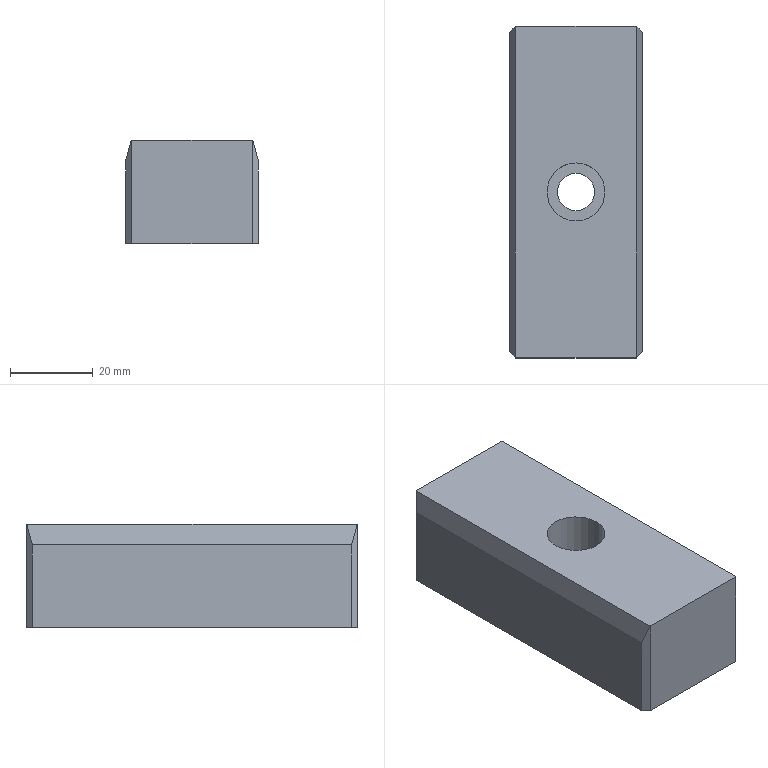Part | NX | features solid 2 | 1 solid | 15 faces | box 32 x 80 x 25 mm | volume 60691 mm3 | plane 13 | cylinder 2 | commonest cylinder face diameters 9 x1 14 x1
STEP:
#1=CARTESIAN_POINT('',(465.,749.5,-145.));
#2=VERTEX_POINT('',#1);
#3=CARTESIAN_POINT('',(465.,745.,-145.));
#4=DIRECTION('',(0.,0.,-1.));
#5=DIRECTION('',(0.,1.,0.));
#6=AXIS2_PLACEMENT_3D('',#3,#4,#5);
#7=CIRCLE('',#6,4.5);
#8=EDGE_CURVE('',#2,#2,#7,.F.);
#9=ORIENTED_EDGE('',*,*,#8,.F.);
#10=EDGE_LOOP('',(#9));
#11=FACE_BOUND('',#10,.T.);
#12=CARTESIAN_POINT('',(465.,740.5,-132.));
#13=VERTEX_POINT('',#12);
#14=CARTESIAN_POINT('',(465.,745.,-132.));
#15=DIRECTION('',(0.,0.,1.));
#16=DIRECTION('',(0.,-1.,0.));
#17=AXIS2_PLACEMENT_3D('',#14,#15,#16);
#18=CIRCLE('',#17,4.5);
#19=EDGE_CURVE('',#13,#13,#18,.T.);
#20=ORIENTED_EDGE('',*,*,#19,.T.);
#21=EDGE_LOOP('',(#20));
#22=FACE_BOUND('',#21,.T.);
#23=CARTESIAN_POINT('',(465.,745.,-70.));
#24=DIRECTION('',(0.,0.,-1.));
#25=DIRECTION('',(0.,1.,0.));
#26=AXIS2_PLACEMENT_3D('',#23,#24,#25);
#27=CYLINDRICAL_SURFACE('',#26,4.5);
#28=ADVANCED_FACE('',(#11,#22),#27,.F.);
#29=CARTESIAN_POINT('',(479.5,705.,-145.));
#30=VERTEX_POINT('',#29);
#31=CARTESIAN_POINT('',(450.5,705.,-145.));
#32=VERTEX_POINT('',#31);
#33=CARTESIAN_POINT('',(481.,705.,-145.));
#34=DIRECTION('',(-1.,0.,0.));
#35=VECTOR('',#34,1000.);
#36=LINE('',#33,#35);
#37=EDGE_CURVE('',#30,#32,#36,.T.);
#38=ORIENTED_EDGE('',*,*,#37,.T.);
#39=CARTESIAN_POINT('',(449.,706.5,-145.));
#40=VERTEX_POINT('',#39);
#41=CARTESIAN_POINT('',(425.75,729.75,-145.));
#42=DIRECTION('',(0.7071,-0.7071,0.));
#43=VECTOR('',#42,1000.);
#44=LINE('',#41,#43);
#45=EDGE_CURVE('',#32,#40,#44,.F.);
#46=ORIENTED_EDGE('',*,*,#45,.T.);
#47=CARTESIAN_POINT('',(449.,783.5,-145.));
#48=VERTEX_POINT('',#47);
#49=CARTESIAN_POINT('',(449.,705.,-145.));
#50=DIRECTION('',(0.,1.,0.));
#51=VECTOR('',#50,1000.);
#52=LINE('',#49,#51);
#53=EDGE_CURVE('',#40,#48,#52,.T.);
#54=ORIENTED_EDGE('',*,*,#53,.T.);
#55=CARTESIAN_POINT('',(450.5,785.,-145.));
#56=VERTEX_POINT('',#55);
#57=CARTESIAN_POINT('',(465.75,800.25,-145.));
#58=DIRECTION('',(-0.7071,-0.7071,0.));
#59=VECTOR('',#58,1000.);
#60=LINE('',#57,#59);
#61=EDGE_CURVE('',#48,#56,#60,.F.);
#62=ORIENTED_EDGE('',*,*,#61,.T.);
#63=CARTESIAN_POINT('',(479.5,785.,-145.));
#64=VERTEX_POINT('',#63);
#65=CARTESIAN_POINT('',(449.,785.,-145.));
#66=DIRECTION('',(1.,0.,0.));
#67=VECTOR('',#66,1000.);
#68=LINE('',#65,#67);
#69=EDGE_CURVE('',#56,#64,#68,.T.);
#70=ORIENTED_EDGE('',*,*,#69,.T.);
#71=CARTESIAN_POINT('',(481.,783.5,-145.));
#72=VERTEX_POINT('',#71);
#73=CARTESIAN_POINT('',(480.25,784.25,-145.));
#74=DIRECTION('',(-0.7071,0.7071,0.));
#75=VECTOR('',#74,1000.);
#76=LINE('',#73,#75);
#77=EDGE_CURVE('',#64,#72,#76,.F.);
#78=ORIENTED_EDGE('',*,*,#77,.T.);
#79=CARTESIAN_POINT('',(481.,706.5,-145.));
#80=VERTEX_POINT('',#79);
#81=CARTESIAN_POINT('',(481.,785.,-145.));
#82=DIRECTION('',(0.,-1.,0.));
#83=VECTOR('',#82,1000.);
#84=LINE('',#81,#83);
#85=EDGE_CURVE('',#72,#80,#84,.T.);
#86=ORIENTED_EDGE('',*,*,#85,.T.);
#87=CARTESIAN_POINT('',(520.25,745.75,-145.));
#88=DIRECTION('',(0.7071,0.7071,0.));
#89=VECTOR('',#88,1000.);
#90=LINE('',#87,#89);
#91=EDGE_CURVE('',#80,#30,#90,.F.);
#92=ORIENTED_EDGE('',*,*,#91,.T.);
#93=EDGE_LOOP('',(#38,#46,#54,#62,#70,#78,#86,#92));
#94=FACE_BOUND('',#93,.T.);
#95=ORIENTED_EDGE('',*,*,#8,.T.);
#96=EDGE_LOOP('',(#95));
#97=FACE_BOUND('',#96,.T.);
#98=CARTESIAN_POINT('',(481.,785.,-145.));
#99=DIRECTION('',(0.,0.,-1.));
#100=DIRECTION('',(0.,1.,0.));
#101=AXIS2_PLACEMENT_3D('',#98,#99,#100);
#102=PLANE('',#101);
#103=ADVANCED_FACE('',(#94,#97),#102,.T.);
#104=CARTESIAN_POINT('',(465.,738.,-120.));
#105=VERTEX_POINT('',#104);
#106=CARTESIAN_POINT('',(465.,745.,-120.));
#107=DIRECTION('',(0.,0.,1.));
#108=DIRECTION('',(0.,-1.,0.));
#109=AXIS2_PLACEMENT_3D('',#106,#107,#108);
#110=CIRCLE('',#109,7.);
#111=EDGE_CURVE('',#105,#105,#110,.T.);
#112=ORIENTED_EDGE('',*,*,#111,.F.);
#113=EDGE_LOOP('',(#112));
#114=FACE_BOUND('',#113,.T.);
#115=CARTESIAN_POINT('',(450.5,785.,-120.));
#116=VERTEX_POINT('',#115);
#117=CARTESIAN_POINT('',(450.34,784.84,-120.));
#118=VERTEX_POINT('',#117);
#119=CARTESIAN_POINT('',(450.5,785.,-120.));
#120=DIRECTION('',(0.7071,0.7071,0.));
#121=VECTOR('',#120,1000.);
#122=LINE('',#119,#121);
#123=EDGE_CURVE('',#116,#118,#122,.F.);
#124=ORIENTED_EDGE('',*,*,#123,.T.);
#125=CARTESIAN_POINT('',(450.34,705.16,-120.));
#126=VERTEX_POINT('',#125);
#127=CARTESIAN_POINT('',(450.34,785.,-120.));
#128=DIRECTION('',(0.,-1.,0.));
#129=VECTOR('',#128,1000.);
#130=LINE('',#127,#129);
#131=EDGE_CURVE('',#118,#126,#130,.T.);
#132=ORIENTED_EDGE('',*,*,#131,.T.);
#133=CARTESIAN_POINT('',(450.5,705.,-120.));
#134=VERTEX_POINT('',#133);
#135=CARTESIAN_POINT('',(449.,706.5,-120.));
#136=DIRECTION('',(-0.7071,0.7071,0.));
#137=VECTOR('',#136,1000.);
#138=LINE('',#135,#137);
#139=EDGE_CURVE('',#126,#134,#138,.F.);
#140=ORIENTED_EDGE('',*,*,#139,.T.);
#141=CARTESIAN_POINT('',(479.5,705.,-120.));
#142=VERTEX_POINT('',#141);
#143=CARTESIAN_POINT('',(481.,705.,-120.));
#144=DIRECTION('',(-1.,0.,0.));
#145=VECTOR('',#144,1000.);
#146=LINE('',#143,#145);
#147=EDGE_CURVE('',#142,#134,#146,.T.);
#148=ORIENTED_EDGE('',*,*,#147,.F.);
#149=CARTESIAN_POINT('',(479.66,705.16,-120.));
#150=VERTEX_POINT('',#149);
#151=CARTESIAN_POINT('',(479.5,705.,-120.));
#152=DIRECTION('',(-0.7071,-0.7071,0.));
#153=VECTOR('',#152,1000.);
#154=LINE('',#151,#153);
#155=EDGE_CURVE('',#142,#150,#154,.F.);
#156=ORIENTED_EDGE('',*,*,#155,.T.);
#157=CARTESIAN_POINT('',(479.66,784.84,-120.));
#158=VERTEX_POINT('',#157);
#159=CARTESIAN_POINT('',(479.66,785.,-120.));
#160=DIRECTION('',(0.,1.,0.));
#161=VECTOR('',#160,1000.);
#162=LINE('',#159,#161);
#163=EDGE_CURVE('',#150,#158,#162,.T.);
#164=ORIENTED_EDGE('',*,*,#163,.T.);
#165=CARTESIAN_POINT('',(479.5,785.,-120.));
#166=VERTEX_POINT('',#165);
#167=CARTESIAN_POINT('',(481.,783.5,-120.));
#168=DIRECTION('',(0.7071,-0.7071,0.));
#169=VECTOR('',#168,1000.);
#170=LINE('',#167,#169);
#171=EDGE_CURVE('',#158,#166,#170,.F.);
#172=ORIENTED_EDGE('',*,*,#171,.T.);
#173=CARTESIAN_POINT('',(449.,785.,-120.));
#174=DIRECTION('',(1.,0.,0.));
#175=VECTOR('',#174,1000.);
#176=LINE('',#173,#175);
#177=EDGE_CURVE('',#116,#166,#176,.T.);
#178=ORIENTED_EDGE('',*,*,#177,.F.);
#179=EDGE_LOOP('',(#124,#132,#140,#148,#156,#164,#172,#178));
#180=FACE_BOUND('',#179,.T.);
#181=CARTESIAN_POINT('',(481.,785.,-120.));
#182=DIRECTION('',(0.,0.,-1.));
#183=DIRECTION('',(0.,1.,0.));
#184=AXIS2_PLACEMENT_3D('',#181,#182,#183);
#185=PLANE('',#184);
#186=ADVANCED_FACE('',(#114,#180),#185,.F.);
#187=ORIENTED_EDGE('',*,*,#69,.F.);
#188=CARTESIAN_POINT('',(450.5,785.,-145.));
#189=DIRECTION('',(0.,0.,1.));
#190=VECTOR('',#189,1000.);
#191=LINE('',#188,#190);
#192=EDGE_CURVE('',#56,#116,#191,.T.);
#193=ORIENTED_EDGE('',*,*,#192,.T.);
#194=ORIENTED_EDGE('',*,*,#177,.T.);
#195=CARTESIAN_POINT('',(479.5,785.,-145.));
#196=DIRECTION('',(0.,0.,-1.));
#197=VECTOR('',#196,1000.);
#198=LINE('',#195,#197);
#199=EDGE_CURVE('',#166,#64,#198,.T.);
#200=ORIENTED_EDGE('',*,*,#199,.T.);
#201=EDGE_LOOP('',(#187,#193,#194,#200));
#202=FACE_BOUND('',#201,.T.);
#203=CARTESIAN_POINT('',(449.,785.,-145.));
#204=DIRECTION('',(0.,-1.,0.));
#205=DIRECTION('',(0.,0.,-1.));
#206=AXIS2_PLACEMENT_3D('',#203,#204,#205);
#207=PLANE('',#206);
#208=ADVANCED_FACE('',(#202),#207,.F.);
#209=CARTESIAN_POINT('',(481.,783.5,-125.));
#210=VERTEX_POINT('',#209);
#211=CARTESIAN_POINT('',(481.,783.5,-145.));
#212=DIRECTION('',(0.,0.,1.));
#213=VECTOR('',#212,1000.);
#214=LINE('',#211,#213);
#215=EDGE_CURVE('',#72,#210,#214,.T.);
#216=ORIENTED_EDGE('',*,*,#215,.T.);
#217=CARTESIAN_POINT('',(481.,706.5,-125.));
#218=VERTEX_POINT('',#217);
#219=CARTESIAN_POINT('',(481.,785.,-125.));
#220=DIRECTION('',(0.,-1.,0.));
#221=VECTOR('',#220,1000.);
#222=LINE('',#219,#221);
#223=EDGE_CURVE('',#210,#218,#222,.T.);
#224=ORIENTED_EDGE('',*,*,#223,.T.);
#225=CARTESIAN_POINT('',(481.,706.5,-145.));
#226=DIRECTION('',(0.,0.,-1.));
#227=VECTOR('',#226,1000.);
#228=LINE('',#225,#227);
#229=EDGE_CURVE('',#218,#80,#228,.T.);
#230=ORIENTED_EDGE('',*,*,#229,.T.);
#231=ORIENTED_EDGE('',*,*,#85,.F.);
#232=EDGE_LOOP('',(#216,#224,#230,#231));
#233=FACE_BOUND('',#232,.T.);
#234=CARTESIAN_POINT('',(481.,785.,-145.));
#235=DIRECTION('',(-1.,0.,0.));
#236=DIRECTION('',(0.,0.,-1.));
#237=AXIS2_PLACEMENT_3D('',#234,#235,#236);
#238=PLANE('',#237);
#239=ADVANCED_FACE('',(#233),#238,.F.);
#240=ORIENTED_EDGE('',*,*,#147,.T.);
#241=CARTESIAN_POINT('',(450.5,705.,-145.));
#242=DIRECTION('',(0.,0.,-1.));
#243=VECTOR('',#242,1000.);
#244=LINE('',#241,#243);
#245=EDGE_CURVE('',#134,#32,#244,.T.);
#246=ORIENTED_EDGE('',*,*,#245,.T.);
#247=ORIENTED_EDGE('',*,*,#37,.F.);
#248=CARTESIAN_POINT('',(479.5,705.,-145.));
#249=DIRECTION('',(0.,0.,1.));
#250=VECTOR('',#249,1000.);
#251=LINE('',#248,#250);
#252=EDGE_CURVE('',#30,#142,#251,.T.);
#253=ORIENTED_EDGE('',*,*,#252,.T.);
#254=EDGE_LOOP('',(#240,#246,#247,#253));
#255=FACE_BOUND('',#254,.T.);
#256=CARTESIAN_POINT('',(481.,705.,-145.));
#257=DIRECTION('',(0.,1.,0.));
#258=DIRECTION('',(0.,0.,1.));
#259=AXIS2_PLACEMENT_3D('',#256,#257,#258);
#260=PLANE('',#259);
#261=ADVANCED_FACE('',(#255),#260,.F.);
#262=CARTESIAN_POINT('',(449.,706.5,-125.));
#263=VERTEX_POINT('',#262);
#264=CARTESIAN_POINT('',(449.,706.5,-145.));
#265=DIRECTION('',(0.,0.,1.));
#266=VECTOR('',#265,1000.);
#267=LINE('',#264,#266);
#268=EDGE_CURVE('',#40,#263,#267,.T.);
#269=ORIENTED_EDGE('',*,*,#268,.T.);
#270=CARTESIAN_POINT('',(449.,783.5,-125.));
#271=VERTEX_POINT('',#270);
#272=CARTESIAN_POINT('',(449.,705.,-125.));
#273=DIRECTION('',(0.,1.,0.));
#274=VECTOR('',#273,1000.);
#275=LINE('',#272,#274);
#276=EDGE_CURVE('',#263,#271,#275,.T.);
#277=ORIENTED_EDGE('',*,*,#276,.T.);
#278=CARTESIAN_POINT('',(449.,783.5,-145.));
#279=DIRECTION('',(0.,0.,-1.));
#280=VECTOR('',#279,1000.);
#281=LINE('',#278,#280);
#282=EDGE_CURVE('',#271,#48,#281,.T.);
#283=ORIENTED_EDGE('',*,*,#282,.T.);
#284=ORIENTED_EDGE('',*,*,#53,.F.);
#285=EDGE_LOOP('',(#269,#277,#283,#284));
#286=FACE_BOUND('',#285,.T.);
#287=CARTESIAN_POINT('',(449.,705.,-145.));
#288=DIRECTION('',(1.,0.,0.));
#289=DIRECTION('',(0.,1.,0.));
#290=AXIS2_PLACEMENT_3D('',#287,#288,#289);
#291=PLANE('',#290);
#292=ADVANCED_FACE('',(#286),#291,.F.);
#293=ORIENTED_EDGE('',*,*,#229,.F.);
#294=CARTESIAN_POINT('',(485.498,710.998,-141.786));
#295=DIRECTION('',(-0.2506,-0.2506,0.9351));
#296=VECTOR('',#295,1000.);
#297=LINE('',#294,#296);
#298=EDGE_CURVE('',#218,#150,#297,.T.);
#299=ORIENTED_EDGE('',*,*,#298,.T.);
#300=ORIENTED_EDGE('',*,*,#155,.F.);
#301=ORIENTED_EDGE('',*,*,#252,.F.);
#302=ORIENTED_EDGE('',*,*,#91,.F.);
#303=EDGE_LOOP('',(#293,#299,#300,#301,#302));
#304=FACE_BOUND('',#303,.T.);
#305=CARTESIAN_POINT('',(479.5,705.,-145.));
#306=DIRECTION('',(-0.7071,0.7071,0.));
#307=DIRECTION('',(-0.7071,-0.7071,0.));
#308=AXIS2_PLACEMENT_3D('',#305,#306,#307);
#309=PLANE('',#308);
#310=ADVANCED_FACE('',(#304),#309,.F.);
#311=ORIENTED_EDGE('',*,*,#139,.F.);
#312=CARTESIAN_POINT('',(444.314,711.186,-142.489));
#313=DIRECTION('',(-0.2506,0.2506,-0.9351));
#314=VECTOR('',#313,1000.);
#315=LINE('',#312,#314);
#316=EDGE_CURVE('',#126,#263,#315,.T.);
#317=ORIENTED_EDGE('',*,*,#316,.T.);
#318=ORIENTED_EDGE('',*,*,#268,.F.);
#319=ORIENTED_EDGE('',*,*,#45,.F.);
#320=ORIENTED_EDGE('',*,*,#245,.F.);
#321=EDGE_LOOP('',(#311,#317,#318,#319,#320));
#322=FACE_BOUND('',#321,.T.);
#323=CARTESIAN_POINT('',(449.,706.5,-145.));
#324=DIRECTION('',(0.7071,0.7071,0.));
#325=DIRECTION('',(-0.7071,0.7071,0.));
#326=AXIS2_PLACEMENT_3D('',#323,#324,#325);
#327=PLANE('',#326);
#328=ADVANCED_FACE('',(#322),#327,.F.);
#329=ORIENTED_EDGE('',*,*,#282,.F.);
#330=CARTESIAN_POINT('',(444.502,779.002,-141.786));
#331=DIRECTION('',(0.2506,0.2506,0.9351));
#332=VECTOR('',#331,1000.);
#333=LINE('',#330,#332);
#334=EDGE_CURVE('',#271,#118,#333,.T.);
#335=ORIENTED_EDGE('',*,*,#334,.T.);
#336=ORIENTED_EDGE('',*,*,#123,.F.);
#337=ORIENTED_EDGE('',*,*,#192,.F.);
#338=ORIENTED_EDGE('',*,*,#61,.F.);
#339=EDGE_LOOP('',(#329,#335,#336,#337,#338));
#340=FACE_BOUND('',#339,.T.);
#341=CARTESIAN_POINT('',(450.5,785.,-145.));
#342=DIRECTION('',(0.7071,-0.7071,0.));
#343=DIRECTION('',(0.7071,0.7071,0.));
#344=AXIS2_PLACEMENT_3D('',#341,#342,#343);
#345=PLANE('',#344);
#346=ADVANCED_FACE('',(#340),#345,.F.);
#347=ORIENTED_EDGE('',*,*,#171,.F.);
#348=CARTESIAN_POINT('',(485.686,778.814,-142.489));
#349=DIRECTION('',(0.2506,-0.2506,-0.9351));
#350=VECTOR('',#349,1000.);
#351=LINE('',#348,#350);
#352=EDGE_CURVE('',#158,#210,#351,.T.);
#353=ORIENTED_EDGE('',*,*,#352,.T.);
#354=ORIENTED_EDGE('',*,*,#215,.F.);
#355=ORIENTED_EDGE('',*,*,#77,.F.);
#356=ORIENTED_EDGE('',*,*,#199,.F.);
#357=EDGE_LOOP('',(#347,#353,#354,#355,#356));
#358=FACE_BOUND('',#357,.T.);
#359=CARTESIAN_POINT('',(481.,783.5,-145.));
#360=DIRECTION('',(-0.7071,-0.7071,0.));
#361=DIRECTION('',(0.7071,-0.7071,0.));
#362=AXIS2_PLACEMENT_3D('',#359,#360,#361);
#363=PLANE('',#362);
#364=ADVANCED_FACE('',(#358),#363,.F.);
#365=ORIENTED_EDGE('',*,*,#352,.F.);
#366=ORIENTED_EDGE('',*,*,#163,.F.);
#367=ORIENTED_EDGE('',*,*,#298,.F.);
#368=ORIENTED_EDGE('',*,*,#223,.F.);
#369=EDGE_LOOP('',(#365,#366,#367,#368));
#370=FACE_BOUND('',#369,.T.);
#371=CARTESIAN_POINT('',(481.,785.,-125.));
#372=DIRECTION('',(-0.9659,0.,-0.2588));
#373=DIRECTION('',(0.2588,0.,-0.9659));
#374=AXIS2_PLACEMENT_3D('',#371,#372,#373);
#375=PLANE('',#374);
#376=ADVANCED_FACE('',(#370),#375,.F.);
#377=ORIENTED_EDGE('',*,*,#316,.F.);
#378=ORIENTED_EDGE('',*,*,#131,.F.);
#379=ORIENTED_EDGE('',*,*,#334,.F.);
#380=ORIENTED_EDGE('',*,*,#276,.F.);
#381=EDGE_LOOP('',(#377,#378,#379,#380));
#382=FACE_BOUND('',#381,.T.);
#383=CARTESIAN_POINT('',(449.,705.,-125.));
#384=DIRECTION('',(0.9659,0.,-0.2588));
#385=DIRECTION('',(0.2588,0.,0.9659));
#386=AXIS2_PLACEMENT_3D('',#383,#384,#385);
#387=PLANE('',#386);
#388=ADVANCED_FACE('',(#382),#387,.F.);
#389=CARTESIAN_POINT('',(465.,738.,-132.));
#390=VERTEX_POINT('',#389);
#391=CARTESIAN_POINT('',(465.,745.,-132.));
#392=DIRECTION('',(0.,0.,1.));
#393=DIRECTION('',(0.,-1.,0.));
#394=AXIS2_PLACEMENT_3D('',#391,#392,#393);
#395=CIRCLE('',#394,7.);
#396=EDGE_CURVE('',#390,#390,#395,.T.);
#397=ORIENTED_EDGE('',*,*,#396,.F.);
#398=EDGE_LOOP('',(#397));
#399=FACE_BOUND('',#398,.T.);
#400=ORIENTED_EDGE('',*,*,#111,.T.);
#401=EDGE_LOOP('',(#400));
#402=FACE_BOUND('',#401,.T.);
#403=CARTESIAN_POINT('',(465.,745.,-132.));
#404=DIRECTION('',(0.,0.,1.));
#405=DIRECTION('',(0.,-1.,0.));
#406=AXIS2_PLACEMENT_3D('',#403,#404,#405);
#407=CYLINDRICAL_SURFACE('',#406,7.);
#408=ADVANCED_FACE('',(#399,#402),#407,.F.);
#409=ORIENTED_EDGE('',*,*,#19,.F.);
#410=EDGE_LOOP('',(#409));
#411=FACE_BOUND('',#410,.T.);
#412=ORIENTED_EDGE('',*,*,#396,.T.);
#413=EDGE_LOOP('',(#412));
#414=FACE_BOUND('',#413,.T.);
#415=CARTESIAN_POINT('',(465.,745.,-132.));
#416=DIRECTION('',(0.,0.,1.));
#417=DIRECTION('',(0.,-1.,0.));
#418=AXIS2_PLACEMENT_3D('',#415,#416,#417);
#419=PLANE('',#418);
#420=ADVANCED_FACE('',(#411,#414),#419,.T.);
#421=CLOSED_SHELL('',(#28,#103,#186,#208,#239,#261,#292,#310,#328,#346,#364,#376,#388,#408,#420));
#422=MANIFOLD_SOLID_BREP('',#421);
#423=(LENGTH_UNIT()NAMED_UNIT(*)SI_UNIT(.MILLI.,.METRE.));
#424=UNCERTAINTY_MEASURE_WITH_UNIT(LENGTH_MEASURE(0.00001),#423,'','');
#425=(NAMED_UNIT(*)PLANE_ANGLE_UNIT()SI_UNIT($,.RADIAN.));
#426=(NAMED_UNIT(*)SI_UNIT($,.STERADIAN.)SOLID_ANGLE_UNIT());
#427=(GEOMETRIC_REPRESENTATION_CONTEXT(3)GLOBAL_UNCERTAINTY_ASSIGNED_CONTEXT((#424))GLOBAL_UNIT_ASSIGNED_CONTEXT((#423,#425,#426))REPRESENTATION_CONTEXT('',''));
#428=ADVANCED_BREP_SHAPE_REPRESENTATION('',(#422),#427);